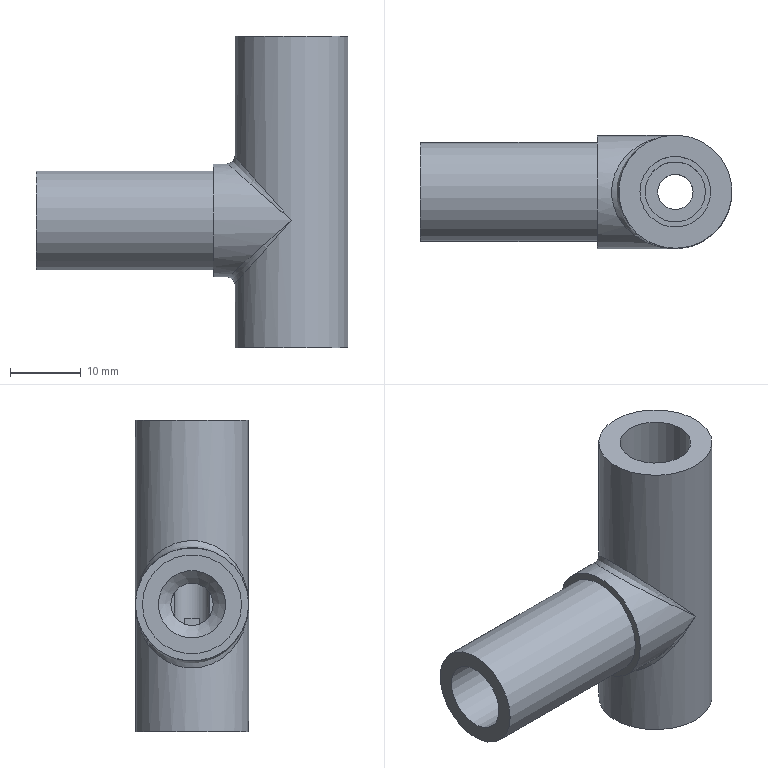Part | STEP file | 1-55.1 | 1 solid | 37 faces | box 44 x 16 x 44 mm | volume 8886 mm3 | plane 24 | cylinder 10 | spline 2 | cone 1 | commonest cylinder face diameters 8.5 x2 10 x2 16 x2 5 x1 6 x1 9.5 x1